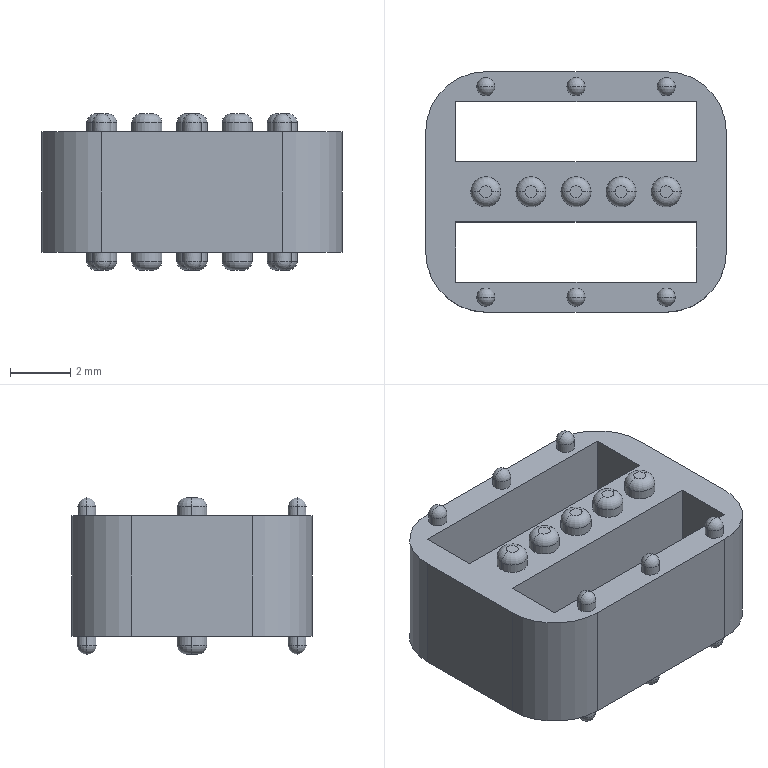Part | SolidWorks | features Fillet 5, ICE 3, Extrusion 1 | 1 solid | 120 faces | box 10 x 8 x 5.2 mm | volume 182.605 mm3 | cylinder 50 | plane 26 | sphere 22 | torus 22 | commonest cylinder face diameters 0.6 x22 1 x20 4 x4 0.65 x2 2 x2